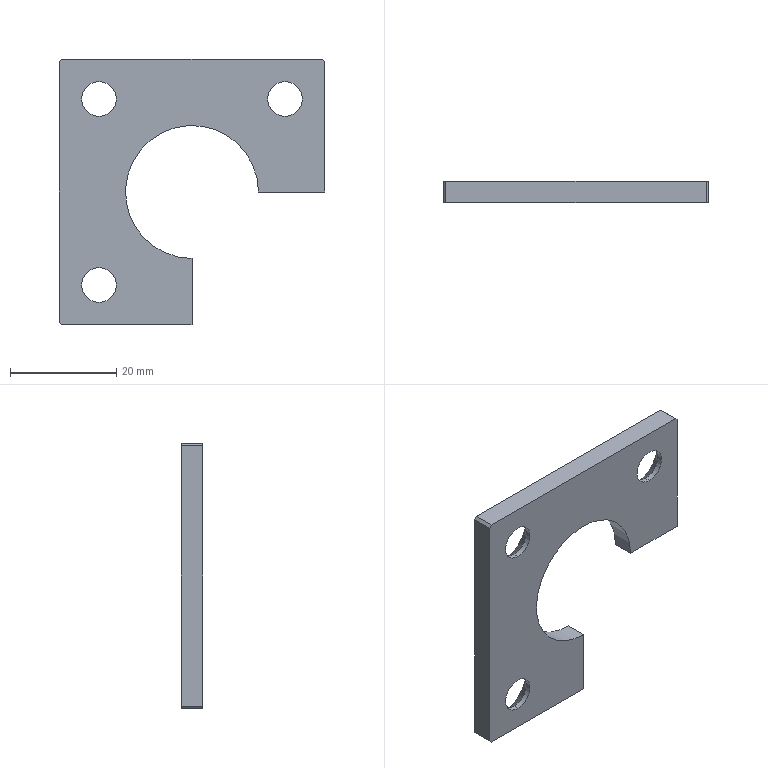Part | STEP file | Cuon T phu H01_4 | 1 solid | 24 faces | box 50 x 4 x 50 mm | volume 5267 mm3 | plane 11 | cylinder 7 | cone 6 | commonest cylinder face diameters 6.5 x6 25 x1